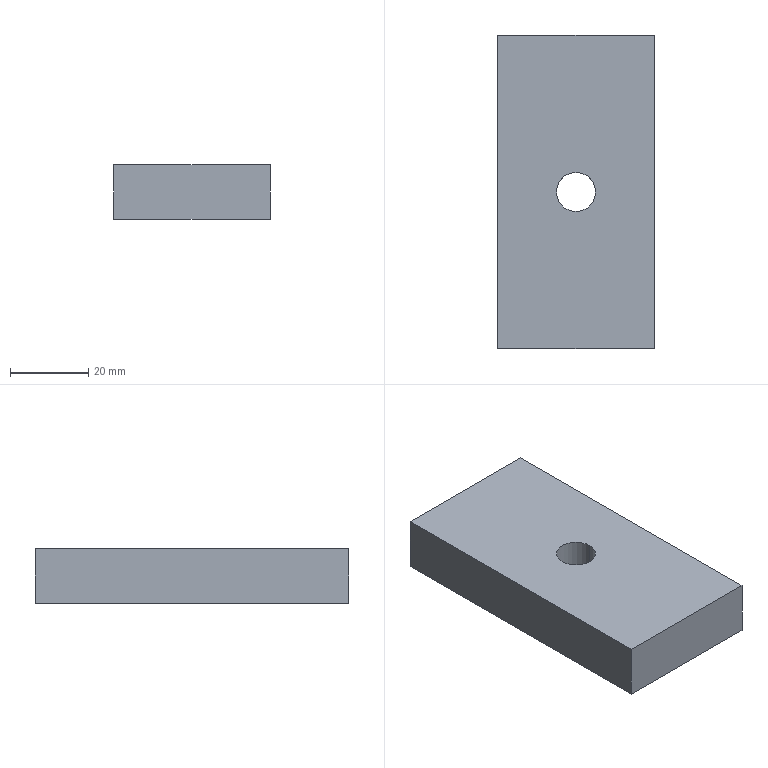Part | SolidWorks | features Extrusion 1, HoleWzd 1 | 1 solid | 8 faces | box 40 x 80 x 14 mm | volume 43700 mm3 | plane 6 | cylinder 2 | commonest cylinder face diameters 10 x2
STEP:
#1=CARTESIAN_POINT('',(15.,40.,14.));
#2=VERTEX_POINT('',#1);
#3=CARTESIAN_POINT('',(25.,40.,14.));
#4=VERTEX_POINT('',#3);
#5=CARTESIAN_POINT('',(20.,40.,14.));
#6=DIRECTION('',(0.,0.,1.));
#7=DIRECTION('',(1.,0.,0.));
#8=AXIS2_PLACEMENT_3D('',#5,#6,#7);
#9=CIRCLE('',#8,5.);
#10=EDGE_CURVE('',#2,#4,#9,.T.);
#11=ORIENTED_EDGE('',*,*,#10,.T.);
#12=CARTESIAN_POINT('',(25.,40.,0.));
#13=VERTEX_POINT('',#12);
#14=CARTESIAN_POINT('',(25.,40.,14.));
#15=DIRECTION('',(0.,0.,-1.));
#16=VECTOR('',#15,1000.);
#17=LINE('',#14,#16);
#18=EDGE_CURVE('',#4,#13,#17,.T.);
#19=ORIENTED_EDGE('',*,*,#18,.T.);
#20=CARTESIAN_POINT('',(15.,40.,0.));
#21=VERTEX_POINT('',#20);
#22=CARTESIAN_POINT('',(20.,40.,0.));
#23=DIRECTION('',(0.,0.,1.));
#24=DIRECTION('',(1.,0.,0.));
#25=AXIS2_PLACEMENT_3D('',#22,#23,#24);
#26=CIRCLE('',#25,5.);
#27=EDGE_CURVE('',#21,#13,#26,.T.);
#28=ORIENTED_EDGE('',*,*,#27,.F.);
#29=CARTESIAN_POINT('',(15.,40.,14.));
#30=DIRECTION('',(0.,0.,-1.));
#31=VECTOR('',#30,1000.);
#32=LINE('',#29,#31);
#33=EDGE_CURVE('',#2,#21,#32,.T.);
#34=ORIENTED_EDGE('',*,*,#33,.F.);
#35=EDGE_LOOP('',(#11,#19,#28,#34));
#36=FACE_OUTER_BOUND('',#35,.T.);
#37=CARTESIAN_POINT('',(20.,40.,14.));
#38=DIRECTION('',(0.,0.,-1.));
#39=DIRECTION('',(-1.,0.,0.));
#40=AXIS2_PLACEMENT_3D('',#37,#38,#39);
#41=CYLINDRICAL_SURFACE('',#40,5.);
#42=ADVANCED_FACE('',(#36),#41,.F.);
#43=CARTESIAN_POINT('',(0.,80.,14.));
#44=VERTEX_POINT('',#43);
#45=CARTESIAN_POINT('',(0.,0.,14.));
#46=VERTEX_POINT('',#45);
#47=CARTESIAN_POINT('',(0.,80.,14.));
#48=DIRECTION('',(0.,-1.,0.));
#49=VECTOR('',#48,1000.);
#50=LINE('',#47,#49);
#51=EDGE_CURVE('',#44,#46,#50,.T.);
#52=ORIENTED_EDGE('',*,*,#51,.T.);
#53=CARTESIAN_POINT('',(40.,0.,14.));
#54=VERTEX_POINT('',#53);
#55=CARTESIAN_POINT('',(0.,0.,14.));
#56=DIRECTION('',(1.,0.,0.));
#57=VECTOR('',#56,1000.);
#58=LINE('',#55,#57);
#59=EDGE_CURVE('',#46,#54,#58,.T.);
#60=ORIENTED_EDGE('',*,*,#59,.T.);
#61=CARTESIAN_POINT('',(40.,80.,14.));
#62=VERTEX_POINT('',#61);
#63=CARTESIAN_POINT('',(40.,0.,14.));
#64=DIRECTION('',(0.,1.,0.));
#65=VECTOR('',#64,1000.);
#66=LINE('',#63,#65);
#67=EDGE_CURVE('',#54,#62,#66,.T.);
#68=ORIENTED_EDGE('',*,*,#67,.T.);
#69=CARTESIAN_POINT('',(40.,80.,14.));
#70=DIRECTION('',(-1.,0.,0.));
#71=VECTOR('',#70,1000.);
#72=LINE('',#69,#71);
#73=EDGE_CURVE('',#62,#44,#72,.T.);
#74=ORIENTED_EDGE('',*,*,#73,.T.);
#75=EDGE_LOOP('',(#52,#60,#68,#74));
#76=FACE_OUTER_BOUND('',#75,.T.);
#77=ORIENTED_EDGE('',*,*,#10,.F.);
#78=CARTESIAN_POINT('',(20.,40.,14.));
#79=DIRECTION('',(0.,0.,1.));
#80=DIRECTION('',(1.,0.,0.));
#81=AXIS2_PLACEMENT_3D('',#78,#79,#80);
#82=CIRCLE('',#81,5.);
#83=EDGE_CURVE('',#4,#2,#82,.T.);
#84=ORIENTED_EDGE('',*,*,#83,.F.);
#85=EDGE_LOOP('',(#77,#84));
#86=FACE_BOUND('',#85,.T.);
#87=CARTESIAN_POINT('',(0.,0.,14.));
#88=DIRECTION('',(0.,0.,1.));
#89=DIRECTION('',(1.,0.,0.));
#90=AXIS2_PLACEMENT_3D('',#87,#88,#89);
#91=PLANE('',#90);
#92=ADVANCED_FACE('',(#76,#86),#91,.T.);
#93=CARTESIAN_POINT('',(0.,80.,0.));
#94=VERTEX_POINT('',#93);
#95=CARTESIAN_POINT('',(0.,0.,0.));
#96=VERTEX_POINT('',#95);
#97=CARTESIAN_POINT('',(0.,80.,0.));
#98=DIRECTION('',(0.,-1.,0.));
#99=VECTOR('',#98,1000.);
#100=LINE('',#97,#99);
#101=EDGE_CURVE('',#94,#96,#100,.T.);
#102=ORIENTED_EDGE('',*,*,#101,.F.);
#103=CARTESIAN_POINT('',(40.,80.,0.));
#104=VERTEX_POINT('',#103);
#105=CARTESIAN_POINT('',(40.,80.,0.));
#106=DIRECTION('',(-1.,0.,0.));
#107=VECTOR('',#106,1000.);
#108=LINE('',#105,#107);
#109=EDGE_CURVE('',#104,#94,#108,.T.);
#110=ORIENTED_EDGE('',*,*,#109,.F.);
#111=CARTESIAN_POINT('',(40.,0.,0.));
#112=VERTEX_POINT('',#111);
#113=CARTESIAN_POINT('',(40.,0.,0.));
#114=DIRECTION('',(0.,1.,0.));
#115=VECTOR('',#114,1000.);
#116=LINE('',#113,#115);
#117=EDGE_CURVE('',#112,#104,#116,.T.);
#118=ORIENTED_EDGE('',*,*,#117,.F.);
#119=CARTESIAN_POINT('',(0.,0.,0.));
#120=DIRECTION('',(1.,0.,0.));
#121=VECTOR('',#120,1000.);
#122=LINE('',#119,#121);
#123=EDGE_CURVE('',#96,#112,#122,.T.);
#124=ORIENTED_EDGE('',*,*,#123,.F.);
#125=EDGE_LOOP('',(#102,#110,#118,#124));
#126=FACE_OUTER_BOUND('',#125,.T.);
#127=ORIENTED_EDGE('',*,*,#27,.T.);
#128=CARTESIAN_POINT('',(20.,40.,0.));
#129=DIRECTION('',(0.,0.,1.));
#130=DIRECTION('',(1.,0.,0.));
#131=AXIS2_PLACEMENT_3D('',#128,#129,#130);
#132=CIRCLE('',#131,5.);
#133=EDGE_CURVE('',#13,#21,#132,.T.);
#134=ORIENTED_EDGE('',*,*,#133,.T.);
#135=EDGE_LOOP('',(#127,#134));
#136=FACE_BOUND('',#135,.T.);
#137=CARTESIAN_POINT('',(0.,0.,0.));
#138=DIRECTION('',(0.,0.,1.));
#139=DIRECTION('',(1.,0.,0.));
#140=AXIS2_PLACEMENT_3D('',#137,#138,#139);
#141=PLANE('',#140);
#142=ADVANCED_FACE('',(#126,#136),#141,.F.);
#143=ORIENTED_EDGE('',*,*,#101,.T.);
#144=CARTESIAN_POINT('',(0.,0.,14.));
#145=DIRECTION('',(0.,0.,-1.));
#146=VECTOR('',#145,1000.);
#147=LINE('',#144,#146);
#148=EDGE_CURVE('',#46,#96,#147,.T.);
#149=ORIENTED_EDGE('',*,*,#148,.F.);
#150=ORIENTED_EDGE('',*,*,#51,.F.);
#151=CARTESIAN_POINT('',(0.,80.,14.));
#152=DIRECTION('',(0.,0.,-1.));
#153=VECTOR('',#152,1000.);
#154=LINE('',#151,#153);
#155=EDGE_CURVE('',#44,#94,#154,.T.);
#156=ORIENTED_EDGE('',*,*,#155,.T.);
#157=EDGE_LOOP('',(#143,#149,#150,#156));
#158=FACE_OUTER_BOUND('',#157,.T.);
#159=CARTESIAN_POINT('',(0.,80.,14.));
#160=DIRECTION('',(1.,0.,0.));
#161=DIRECTION('',(0.,1.,0.));
#162=AXIS2_PLACEMENT_3D('',#159,#160,#161);
#163=PLANE('',#162);
#164=ADVANCED_FACE('',(#158),#163,.F.);
#165=ORIENTED_EDGE('',*,*,#123,.T.);
#166=CARTESIAN_POINT('',(40.,0.,14.));
#167=DIRECTION('',(0.,0.,-1.));
#168=VECTOR('',#167,1000.);
#169=LINE('',#166,#168);
#170=EDGE_CURVE('',#54,#112,#169,.T.);
#171=ORIENTED_EDGE('',*,*,#170,.F.);
#172=ORIENTED_EDGE('',*,*,#59,.F.);
#173=ORIENTED_EDGE('',*,*,#148,.T.);
#174=EDGE_LOOP('',(#165,#171,#172,#173));
#175=FACE_OUTER_BOUND('',#174,.T.);
#176=CARTESIAN_POINT('',(0.,0.,14.));
#177=DIRECTION('',(0.,1.,0.));
#178=DIRECTION('',(0.,0.,1.));
#179=AXIS2_PLACEMENT_3D('',#176,#177,#178);
#180=PLANE('',#179);
#181=ADVANCED_FACE('',(#175),#180,.F.);
#182=ORIENTED_EDGE('',*,*,#117,.T.);
#183=CARTESIAN_POINT('',(40.,80.,14.));
#184=DIRECTION('',(0.,0.,-1.));
#185=VECTOR('',#184,1000.);
#186=LINE('',#183,#185);
#187=EDGE_CURVE('',#62,#104,#186,.T.);
#188=ORIENTED_EDGE('',*,*,#187,.F.);
#189=ORIENTED_EDGE('',*,*,#67,.F.);
#190=ORIENTED_EDGE('',*,*,#170,.T.);
#191=EDGE_LOOP('',(#182,#188,#189,#190));
#192=FACE_OUTER_BOUND('',#191,.T.);
#193=CARTESIAN_POINT('',(40.,0.,14.));
#194=DIRECTION('',(-1.,0.,0.));
#195=DIRECTION('',(0.,0.,1.));
#196=AXIS2_PLACEMENT_3D('',#193,#194,#195);
#197=PLANE('',#196);
#198=ADVANCED_FACE('',(#192),#197,.F.);
#199=ORIENTED_EDGE('',*,*,#109,.T.);
#200=ORIENTED_EDGE('',*,*,#155,.F.);
#201=ORIENTED_EDGE('',*,*,#73,.F.);
#202=ORIENTED_EDGE('',*,*,#187,.T.);
#203=EDGE_LOOP('',(#199,#200,#201,#202));
#204=FACE_OUTER_BOUND('',#203,.T.);
#205=CARTESIAN_POINT('',(40.,80.,14.));
#206=DIRECTION('',(0.,-1.,0.));
#207=DIRECTION('',(1.,0.,0.));
#208=AXIS2_PLACEMENT_3D('',#205,#206,#207);
#209=PLANE('',#208);
#210=ADVANCED_FACE('',(#204),#209,.F.);
#211=ORIENTED_EDGE('',*,*,#18,.F.);
#212=ORIENTED_EDGE('',*,*,#83,.T.);
#213=ORIENTED_EDGE('',*,*,#33,.T.);
#214=ORIENTED_EDGE('',*,*,#133,.F.);
#215=EDGE_LOOP('',(#211,#212,#213,#214));
#216=FACE_OUTER_BOUND('',#215,.T.);
#217=CARTESIAN_POINT('',(20.,40.,14.));
#218=DIRECTION('',(0.,0.,-1.));
#219=DIRECTION('',(-1.,0.,0.));
#220=AXIS2_PLACEMENT_3D('',#217,#218,#219);
#221=CYLINDRICAL_SURFACE('',#220,5.);
#222=ADVANCED_FACE('',(#216),#221,.F.);
#223=CLOSED_SHELL('',(#42,#92,#142,#164,#181,#198,#210,#222));
#224=MANIFOLD_SOLID_BREP('',#223);
#225=CARTESIAN_POINT('',(0.,0.,0.));
#226=DIRECTION('',(0.,0.,1.));
#227=DIRECTION('',(1.,0.,0.));
#228=AXIS2_PLACEMENT_3D('',#225,#226,#227);
#229=(LENGTH_UNIT()NAMED_UNIT(*)SI_UNIT(.MILLI.,.METRE.));
#230=UNCERTAINTY_MEASURE_WITH_UNIT(LENGTH_MEASURE(0.00001),#229,'','');
#231=(NAMED_UNIT(*)PLANE_ANGLE_UNIT()SI_UNIT($,.RADIAN.));
#232=(NAMED_UNIT(*)SI_UNIT($,.STERADIAN.)SOLID_ANGLE_UNIT());
#233=(GEOMETRIC_REPRESENTATION_CONTEXT(3)GLOBAL_UNCERTAINTY_ASSIGNED_CONTEXT((#230))GLOBAL_UNIT_ASSIGNED_CONTEXT((#229,#231,#232))REPRESENTATION_CONTEXT('',''));
#234=ADVANCED_BREP_SHAPE_REPRESENTATION('',(#224,#228),#233);